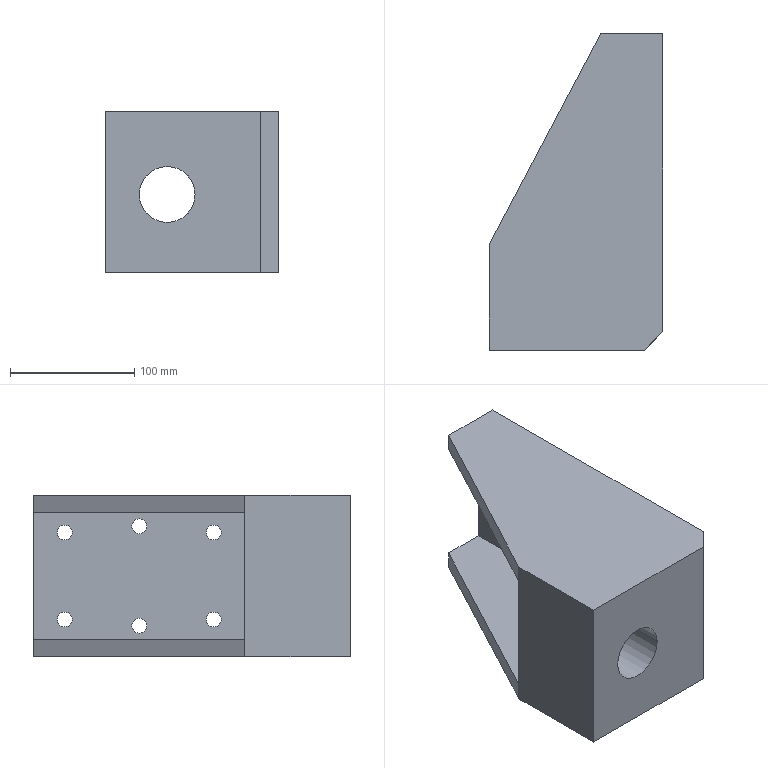Part | SolidWorks | features ICE 4, HoleWzd 2, Extrusion 1 | 1 solid | 27 faces | box 140 x 255 x 130 mm | volume 2115971 mm3 | cylinder 14 | plane 13 | commonest cylinder face diameters 12 x12 45 x2
STEP:
#1=CARTESIAN_POINT('',(-67.5,90.,63.));
#2=VERTEX_POINT('',#1);
#3=CARTESIAN_POINT('',(-112.5,90.,63.));
#4=VERTEX_POINT('',#3);
#5=CARTESIAN_POINT('',(-90.,90.,63.));
#6=DIRECTION('',(0.,1.,0.));
#7=DIRECTION('',(0.,0.,1.));
#8=AXIS2_PLACEMENT_3D('',#5,#6,#7);
#9=CIRCLE('',#8,22.5);
#10=EDGE_CURVE('',#2,#4,#9,.T.);
#11=ORIENTED_EDGE('',*,*,#10,.T.);
#12=CARTESIAN_POINT('',(-112.5,5.,63.));
#13=VERTEX_POINT('',#12);
#14=CARTESIAN_POINT('',(-112.5,260.001,63.));
#15=DIRECTION('',(0.,-1.,0.));
#16=VECTOR('',#15,1000.);
#17=LINE('',#14,#16);
#18=EDGE_CURVE('',#4,#13,#17,.T.);
#19=ORIENTED_EDGE('',*,*,#18,.T.);
#20=CARTESIAN_POINT('',(-67.5,5.,63.));
#21=VERTEX_POINT('',#20);
#22=CARTESIAN_POINT('',(-90.,5.,63.));
#23=DIRECTION('',(0.,1.,0.));
#24=DIRECTION('',(-1.,0.,0.));
#25=AXIS2_PLACEMENT_3D('',#22,#23,#24);
#26=CIRCLE('',#25,22.5);
#27=EDGE_CURVE('',#21,#13,#26,.T.);
#28=ORIENTED_EDGE('',*,*,#27,.F.);
#29=CARTESIAN_POINT('',(-67.5,260.001,63.));
#30=DIRECTION('',(0.,-1.,0.));
#31=VECTOR('',#30,1000.);
#32=LINE('',#29,#31);
#33=EDGE_CURVE('',#2,#21,#32,.T.);
#34=ORIENTED_EDGE('',*,*,#33,.F.);
#35=EDGE_LOOP('',(#11,#19,#28,#34));
#36=FACE_OUTER_BOUND('',#35,.T.);
#37=CARTESIAN_POINT('',(-90.,260.001,63.));
#38=DIRECTION('',(0.,-1.,0.));
#39=DIRECTION('',(1.,0.,0.));
#40=AXIS2_PLACEMENT_3D('',#37,#38,#39);
#41=CYLINDRICAL_SURFACE('',#40,22.5);
#42=ADVANCED_FACE('',(#36),#41,.F.);
#43=CARTESIAN_POINT('',(-16.,175.,99.));
#44=VERTEX_POINT('',#43);
#45=CARTESIAN_POINT('',(-16.,175.,111.));
#46=VERTEX_POINT('',#45);
#47=CARTESIAN_POINT('',(-16.,175.,105.));
#48=DIRECTION('',(-1.,0.,0.));
#49=DIRECTION('',(0.,-1.,0.));
#50=AXIS2_PLACEMENT_3D('',#47,#48,#49);
#51=CIRCLE('',#50,6.);
#52=EDGE_CURVE('',#44,#46,#51,.T.);
#53=ORIENTED_EDGE('',*,*,#52,.T.);
#54=CARTESIAN_POINT('',(0.,175.,111.));
#55=VERTEX_POINT('',#54);
#56=CARTESIAN_POINT('',(0.,175.,111.));
#57=DIRECTION('',(1.,0.,0.));
#58=VECTOR('',#57,1000.);
#59=LINE('',#56,#58);
#60=EDGE_CURVE('',#46,#55,#59,.T.);
#61=ORIENTED_EDGE('',*,*,#60,.T.);
#62=CARTESIAN_POINT('',(0.,175.,99.));
#63=VERTEX_POINT('',#62);
#64=CARTESIAN_POINT('',(0.,175.,105.));
#65=DIRECTION('',(1.,0.,0.));
#66=DIRECTION('',(0.,0.,-1.));
#67=AXIS2_PLACEMENT_3D('',#64,#65,#66);
#68=CIRCLE('',#67,6.);
#69=EDGE_CURVE('',#55,#63,#68,.T.);
#70=ORIENTED_EDGE('',*,*,#69,.T.);
#71=CARTESIAN_POINT('',(0.,175.,99.));
#72=DIRECTION('',(1.,0.,0.));
#73=VECTOR('',#72,1000.);
#74=LINE('',#71,#73);
#75=EDGE_CURVE('',#44,#63,#74,.T.);
#76=ORIENTED_EDGE('',*,*,#75,.F.);
#77=EDGE_LOOP('',(#53,#61,#70,#76));
#78=FACE_OUTER_BOUND('',#77,.T.);
#79=CARTESIAN_POINT('',(0.,175.,105.));
#80=DIRECTION('',(1.,0.,0.));
#81=DIRECTION('',(0.,0.,-1.));
#82=AXIS2_PLACEMENT_3D('',#79,#80,#81);
#83=CYLINDRICAL_SURFACE('',#82,6.);
#84=ADVANCED_FACE('',(#78),#83,.F.);
#85=CARTESIAN_POINT('',(-16.,175.,19.));
#86=VERTEX_POINT('',#85);
#87=CARTESIAN_POINT('',(-16.,175.,31.));
#88=VERTEX_POINT('',#87);
#89=CARTESIAN_POINT('',(-16.,175.,25.));
#90=DIRECTION('',(-1.,0.,0.));
#91=DIRECTION('',(0.,-1.,0.));
#92=AXIS2_PLACEMENT_3D('',#89,#90,#91);
#93=CIRCLE('',#92,6.);
#94=EDGE_CURVE('',#86,#88,#93,.T.);
#95=ORIENTED_EDGE('',*,*,#94,.T.);
#96=CARTESIAN_POINT('',(0.,175.,31.));
#97=VERTEX_POINT('',#96);
#98=CARTESIAN_POINT('',(0.,175.,31.));
#99=DIRECTION('',(1.,0.,0.));
#100=VECTOR('',#99,1000.);
#101=LINE('',#98,#100);
#102=EDGE_CURVE('',#88,#97,#101,.T.);
#103=ORIENTED_EDGE('',*,*,#102,.T.);
#104=CARTESIAN_POINT('',(0.,175.,19.));
#105=VERTEX_POINT('',#104);
#106=CARTESIAN_POINT('',(0.,175.,25.));
#107=DIRECTION('',(1.,0.,0.));
#108=DIRECTION('',(0.,0.,-1.));
#109=AXIS2_PLACEMENT_3D('',#106,#107,#108);
#110=CIRCLE('',#109,6.);
#111=EDGE_CURVE('',#97,#105,#110,.T.);
#112=ORIENTED_EDGE('',*,*,#111,.T.);
#113=CARTESIAN_POINT('',(0.,175.,19.));
#114=DIRECTION('',(1.,0.,0.));
#115=VECTOR('',#114,1000.);
#116=LINE('',#113,#115);
#117=EDGE_CURVE('',#86,#105,#116,.T.);
#118=ORIENTED_EDGE('',*,*,#117,.F.);
#119=EDGE_LOOP('',(#95,#103,#112,#118));
#120=FACE_OUTER_BOUND('',#119,.T.);
#121=CARTESIAN_POINT('',(0.,175.,25.));
#122=DIRECTION('',(1.,0.,0.));
#123=DIRECTION('',(0.,0.,-1.));
#124=AXIS2_PLACEMENT_3D('',#121,#122,#123);
#125=CYLINDRICAL_SURFACE('',#124,6.);
#126=ADVANCED_FACE('',(#120),#125,.F.);
#127=CARTESIAN_POINT('',(-16.,235.,94.));
#128=VERTEX_POINT('',#127);
#129=CARTESIAN_POINT('',(-16.,235.,106.));
#130=VERTEX_POINT('',#129);
#131=CARTESIAN_POINT('',(-16.,235.,100.));
#132=DIRECTION('',(-1.,0.,0.));
#133=DIRECTION('',(0.,-1.,0.));
#134=AXIS2_PLACEMENT_3D('',#131,#132,#133);
#135=CIRCLE('',#134,6.);
#136=EDGE_CURVE('',#128,#130,#135,.T.);
#137=ORIENTED_EDGE('',*,*,#136,.T.);
#138=CARTESIAN_POINT('',(0.,235.,106.));
#139=VERTEX_POINT('',#138);
#140=CARTESIAN_POINT('',(0.,235.,106.));
#141=DIRECTION('',(1.,0.,0.));
#142=VECTOR('',#141,1000.);
#143=LINE('',#140,#142);
#144=EDGE_CURVE('',#130,#139,#143,.T.);
#145=ORIENTED_EDGE('',*,*,#144,.T.);
#146=CARTESIAN_POINT('',(0.,235.,94.));
#147=VERTEX_POINT('',#146);
#148=CARTESIAN_POINT('',(0.,235.,100.));
#149=DIRECTION('',(1.,0.,0.));
#150=DIRECTION('',(0.,0.,-1.));
#151=AXIS2_PLACEMENT_3D('',#148,#149,#150);
#152=CIRCLE('',#151,6.);
#153=EDGE_CURVE('',#139,#147,#152,.T.);
#154=ORIENTED_EDGE('',*,*,#153,.T.);
#155=CARTESIAN_POINT('',(0.,235.,94.));
#156=DIRECTION('',(1.,0.,0.));
#157=VECTOR('',#156,1000.);
#158=LINE('',#155,#157);
#159=EDGE_CURVE('',#128,#147,#158,.T.);
#160=ORIENTED_EDGE('',*,*,#159,.F.);
#161=EDGE_LOOP('',(#137,#145,#154,#160));
#162=FACE_OUTER_BOUND('',#161,.T.);
#163=CARTESIAN_POINT('',(0.,235.,100.));
#164=DIRECTION('',(1.,0.,0.));
#165=DIRECTION('',(0.,0.,-1.));
#166=AXIS2_PLACEMENT_3D('',#163,#164,#165);
#167=CYLINDRICAL_SURFACE('',#166,6.);
#168=ADVANCED_FACE('',(#162),#167,.F.);
#169=CARTESIAN_POINT('',(-16.,235.,24.));
#170=VERTEX_POINT('',#169);
#171=CARTESIAN_POINT('',(-16.,235.,36.));
#172=VERTEX_POINT('',#171);
#173=CARTESIAN_POINT('',(-16.,235.,30.));
#174=DIRECTION('',(-1.,0.,0.));
#175=DIRECTION('',(0.,-1.,0.));
#176=AXIS2_PLACEMENT_3D('',#173,#174,#175);
#177=CIRCLE('',#176,6.);
#178=EDGE_CURVE('',#170,#172,#177,.T.);
#179=ORIENTED_EDGE('',*,*,#178,.T.);
#180=CARTESIAN_POINT('',(0.,235.,36.));
#181=VERTEX_POINT('',#180);
#182=CARTESIAN_POINT('',(0.,235.,36.));
#183=DIRECTION('',(1.,0.,0.));
#184=VECTOR('',#183,1000.);
#185=LINE('',#182,#184);
#186=EDGE_CURVE('',#172,#181,#185,.T.);
#187=ORIENTED_EDGE('',*,*,#186,.T.);
#188=CARTESIAN_POINT('',(0.,235.,24.));
#189=VERTEX_POINT('',#188);
#190=CARTESIAN_POINT('',(0.,235.,30.));
#191=DIRECTION('',(1.,0.,0.));
#192=DIRECTION('',(0.,0.,-1.));
#193=AXIS2_PLACEMENT_3D('',#190,#191,#192);
#194=CIRCLE('',#193,6.);
#195=EDGE_CURVE('',#181,#189,#194,.T.);
#196=ORIENTED_EDGE('',*,*,#195,.T.);
#197=CARTESIAN_POINT('',(0.,235.,24.));
#198=DIRECTION('',(1.,0.,0.));
#199=VECTOR('',#198,1000.);
#200=LINE('',#197,#199);
#201=EDGE_CURVE('',#170,#189,#200,.T.);
#202=ORIENTED_EDGE('',*,*,#201,.F.);
#203=EDGE_LOOP('',(#179,#187,#196,#202));
#204=FACE_OUTER_BOUND('',#203,.T.);
#205=CARTESIAN_POINT('',(0.,235.,30.));
#206=DIRECTION('',(1.,0.,0.));
#207=DIRECTION('',(0.,0.,-1.));
#208=AXIS2_PLACEMENT_3D('',#205,#206,#207);
#209=CYLINDRICAL_SURFACE('',#208,6.);
#210=ADVANCED_FACE('',(#204),#209,.F.);
#211=CARTESIAN_POINT('',(-16.,115.,94.));
#212=VERTEX_POINT('',#211);
#213=CARTESIAN_POINT('',(-16.,115.,106.));
#214=VERTEX_POINT('',#213);
#215=CARTESIAN_POINT('',(-16.,115.,100.));
#216=DIRECTION('',(-1.,0.,0.));
#217=DIRECTION('',(0.,-1.,0.));
#218=AXIS2_PLACEMENT_3D('',#215,#216,#217);
#219=CIRCLE('',#218,6.);
#220=EDGE_CURVE('',#212,#214,#219,.T.);
#221=ORIENTED_EDGE('',*,*,#220,.T.);
#222=CARTESIAN_POINT('',(0.,115.,106.));
#223=VERTEX_POINT('',#222);
#224=CARTESIAN_POINT('',(0.,115.,106.));
#225=DIRECTION('',(1.,0.,0.));
#226=VECTOR('',#225,1000.);
#227=LINE('',#224,#226);
#228=EDGE_CURVE('',#214,#223,#227,.T.);
#229=ORIENTED_EDGE('',*,*,#228,.T.);
#230=CARTESIAN_POINT('',(0.,115.,94.));
#231=VERTEX_POINT('',#230);
#232=CARTESIAN_POINT('',(0.,115.,100.));
#233=DIRECTION('',(1.,0.,0.));
#234=DIRECTION('',(0.,0.,-1.));
#235=AXIS2_PLACEMENT_3D('',#232,#233,#234);
#236=CIRCLE('',#235,6.);
#237=EDGE_CURVE('',#223,#231,#236,.T.);
#238=ORIENTED_EDGE('',*,*,#237,.T.);
#239=CARTESIAN_POINT('',(0.,115.,94.));
#240=DIRECTION('',(1.,0.,0.));
#241=VECTOR('',#240,1000.);
#242=LINE('',#239,#241);
#243=EDGE_CURVE('',#212,#231,#242,.T.);
#244=ORIENTED_EDGE('',*,*,#243,.F.);
#245=EDGE_LOOP('',(#221,#229,#238,#244));
#246=FACE_OUTER_BOUND('',#245,.T.);
#247=CARTESIAN_POINT('',(0.,115.,100.));
#248=DIRECTION('',(1.,0.,0.));
#249=DIRECTION('',(0.,0.,-1.));
#250=AXIS2_PLACEMENT_3D('',#247,#248,#249);
#251=CYLINDRICAL_SURFACE('',#250,6.);
#252=ADVANCED_FACE('',(#246),#251,.F.);
#253=CARTESIAN_POINT('',(-16.,115.,24.));
#254=VERTEX_POINT('',#253);
#255=CARTESIAN_POINT('',(-16.,115.,36.));
#256=VERTEX_POINT('',#255);
#257=CARTESIAN_POINT('',(-16.,115.,30.));
#258=DIRECTION('',(-1.,0.,0.));
#259=DIRECTION('',(0.,-1.,0.));
#260=AXIS2_PLACEMENT_3D('',#257,#258,#259);
#261=CIRCLE('',#260,6.);
#262=EDGE_CURVE('',#254,#256,#261,.T.);
#263=ORIENTED_EDGE('',*,*,#262,.T.);
#264=CARTESIAN_POINT('',(0.,115.,36.));
#265=VERTEX_POINT('',#264);
#266=CARTESIAN_POINT('',(0.,115.,36.));
#267=DIRECTION('',(1.,0.,0.));
#268=VECTOR('',#267,1000.);
#269=LINE('',#266,#268);
#270=EDGE_CURVE('',#256,#265,#269,.T.);
#271=ORIENTED_EDGE('',*,*,#270,.T.);
#272=CARTESIAN_POINT('',(0.,115.,24.));
#273=VERTEX_POINT('',#272);
#274=CARTESIAN_POINT('',(0.,115.,30.));
#275=DIRECTION('',(1.,0.,0.));
#276=DIRECTION('',(0.,0.,-1.));
#277=AXIS2_PLACEMENT_3D('',#274,#275,#276);
#278=CIRCLE('',#277,6.);
#279=EDGE_CURVE('',#265,#273,#278,.T.);
#280=ORIENTED_EDGE('',*,*,#279,.T.);
#281=CARTESIAN_POINT('',(0.,115.,24.));
#282=DIRECTION('',(1.,0.,0.));
#283=VECTOR('',#282,1000.);
#284=LINE('',#281,#283);
#285=EDGE_CURVE('',#254,#273,#284,.T.);
#286=ORIENTED_EDGE('',*,*,#285,.F.);
#287=EDGE_LOOP('',(#263,#271,#280,#286));
#288=FACE_OUTER_BOUND('',#287,.T.);
#289=CARTESIAN_POINT('',(0.,115.,30.));
#290=DIRECTION('',(1.,0.,0.));
#291=DIRECTION('',(0.,0.,-1.));
#292=AXIS2_PLACEMENT_3D('',#289,#290,#291);
#293=CYLINDRICAL_SURFACE('',#292,6.);
#294=ADVANCED_FACE('',(#288),#293,.F.);
#295=CARTESIAN_POINT('',(0.,175.,105.));
#296=DIRECTION('',(1.,0.,0.));
#297=DIRECTION('',(0.,0.,-1.));
#298=AXIS2_PLACEMENT_3D('',#295,#296,#297);
#299=CIRCLE('',#298,6.);
#300=EDGE_CURVE('',#63,#55,#299,.T.);
#301=ORIENTED_EDGE('',*,*,#300,.F.);
#302=ORIENTED_EDGE('',*,*,#69,.F.);
#303=EDGE_LOOP('',(#301,#302));
#304=FACE_BOUND('',#303,.T.);
#305=CARTESIAN_POINT('',(0.,235.,100.));
#306=DIRECTION('',(1.,0.,0.));
#307=DIRECTION('',(0.,0.,-1.));
#308=AXIS2_PLACEMENT_3D('',#305,#306,#307);
#309=CIRCLE('',#308,6.);
#310=EDGE_CURVE('',#147,#139,#309,.T.);
#311=ORIENTED_EDGE('',*,*,#310,.F.);
#312=ORIENTED_EDGE('',*,*,#153,.F.);
#313=EDGE_LOOP('',(#311,#312));
#314=FACE_BOUND('',#313,.T.);
#315=CARTESIAN_POINT('',(0.,235.,30.));
#316=DIRECTION('',(1.,0.,0.));
#317=DIRECTION('',(0.,0.,-1.));
#318=AXIS2_PLACEMENT_3D('',#315,#316,#317);
#319=CIRCLE('',#318,6.);
#320=EDGE_CURVE('',#189,#181,#319,.T.);
#321=ORIENTED_EDGE('',*,*,#320,.F.);
#322=ORIENTED_EDGE('',*,*,#195,.F.);
#323=EDGE_LOOP('',(#321,#322));
#324=FACE_BOUND('',#323,.T.);
#325=CARTESIAN_POINT('',(0.,115.,100.));
#326=DIRECTION('',(1.,0.,0.));
#327=DIRECTION('',(0.,0.,-1.));
#328=AXIS2_PLACEMENT_3D('',#325,#326,#327);
#329=CIRCLE('',#328,6.);
#330=EDGE_CURVE('',#231,#223,#329,.T.);
#331=ORIENTED_EDGE('',*,*,#330,.F.);
#332=ORIENTED_EDGE('',*,*,#237,.F.);
#333=EDGE_LOOP('',(#331,#332));
#334=FACE_BOUND('',#333,.T.);
#335=CARTESIAN_POINT('',(0.,115.,30.));
#336=DIRECTION('',(1.,0.,0.));
#337=DIRECTION('',(0.,0.,-1.));
#338=AXIS2_PLACEMENT_3D('',#335,#336,#337);
#339=CIRCLE('',#338,6.);
#340=EDGE_CURVE('',#273,#265,#339,.T.);
#341=ORIENTED_EDGE('',*,*,#340,.F.);
#342=ORIENTED_EDGE('',*,*,#279,.F.);
#343=EDGE_LOOP('',(#341,#342));
#344=FACE_BOUND('',#343,.T.);
#345=CARTESIAN_POINT('',(0.,20.,130.));
#346=VERTEX_POINT('',#345);
#347=CARTESIAN_POINT('',(0.,260.,130.));
#348=VERTEX_POINT('',#347);
#349=CARTESIAN_POINT('',(0.,260.,130.));
#350=DIRECTION('',(0.,1.,0.));
#351=VECTOR('',#350,1000.);
#352=LINE('',#349,#351);
#353=EDGE_CURVE('',#346,#348,#352,.T.);
#354=ORIENTED_EDGE('',*,*,#353,.F.);
#355=CARTESIAN_POINT('',(0.,20.,0.));
#356=VERTEX_POINT('',#355);
#357=CARTESIAN_POINT('',(0.,20.,0.));
#358=DIRECTION('',(0.,0.,1.));
#359=VECTOR('',#358,1000.);
#360=LINE('',#357,#359);
#361=EDGE_CURVE('',#356,#346,#360,.T.);
#362=ORIENTED_EDGE('',*,*,#361,.F.);
#363=CARTESIAN_POINT('',(0.,260.,0.));
#364=VERTEX_POINT('',#363);
#365=CARTESIAN_POINT('',(0.,260.,0.));
#366=DIRECTION('',(0.,1.,0.));
#367=VECTOR('',#366,1000.);
#368=LINE('',#365,#367);
#369=EDGE_CURVE('',#356,#364,#368,.T.);
#370=ORIENTED_EDGE('',*,*,#369,.T.);
#371=CARTESIAN_POINT('',(0.,260.,130.));
#372=DIRECTION('',(0.,0.,-1.));
#373=VECTOR('',#372,1000.);
#374=LINE('',#371,#373);
#375=EDGE_CURVE('',#348,#364,#374,.T.);
#376=ORIENTED_EDGE('',*,*,#375,.F.);
#377=EDGE_LOOP('',(#354,#362,#370,#376));
#378=FACE_OUTER_BOUND('',#377,.T.);
#379=CARTESIAN_POINT('',(0.,175.,25.));
#380=DIRECTION('',(1.,0.,0.));
#381=DIRECTION('',(0.,0.,-1.));
#382=AXIS2_PLACEMENT_3D('',#379,#380,#381);
#383=CIRCLE('',#382,6.);
#384=EDGE_CURVE('',#105,#97,#383,.T.);
#385=ORIENTED_EDGE('',*,*,#384,.F.);
#386=ORIENTED_EDGE('',*,*,#111,.F.);
#387=EDGE_LOOP('',(#385,#386));
#388=FACE_BOUND('',#387,.T.);
#389=CARTESIAN_POINT('',(0.,260.,130.));
#390=DIRECTION('',(-1.,0.,0.));
#391=DIRECTION('',(0.,-1.,0.));
#392=AXIS2_PLACEMENT_3D('',#389,#390,#391);
#393=PLANE('',#392);
#394=ADVANCED_FACE('',(#304,#314,#324,#334,#344,#378,#388),#393,.F.);
#395=CARTESIAN_POINT('',(-16.,260.,14.));
#396=VERTEX_POINT('',#395);
#397=CARTESIAN_POINT('',(-50.,260.,14.));
#398=VERTEX_POINT('',#397);
#399=CARTESIAN_POINT('',(198.252,260.,14.));
#400=DIRECTION('',(-1.,0.,0.));
#401=VECTOR('',#400,1000.);
#402=LINE('',#399,#401);
#403=EDGE_CURVE('',#396,#398,#402,.T.);
#404=ORIENTED_EDGE('',*,*,#403,.F.);
#405=CARTESIAN_POINT('',(-16.,260.,116.));
#406=VERTEX_POINT('',#405);
#407=CARTESIAN_POINT('',(-16.,260.,116.));
#408=DIRECTION('',(0.,0.,-1.));
#409=VECTOR('',#408,1000.);
#410=LINE('',#407,#409);
#411=EDGE_CURVE('',#406,#396,#410,.T.);
#412=ORIENTED_EDGE('',*,*,#411,.F.);
#413=CARTESIAN_POINT('',(-50.,260.,116.));
#414=VERTEX_POINT('',#413);
#415=CARTESIAN_POINT('',(198.252,260.,116.));
#416=DIRECTION('',(-1.,0.,0.));
#417=VECTOR('',#416,1000.);
#418=LINE('',#415,#417);
#419=EDGE_CURVE('',#406,#414,#418,.T.);
#420=ORIENTED_EDGE('',*,*,#419,.T.);
#421=CARTESIAN_POINT('',(-50.,260.,130.));
#422=VERTEX_POINT('',#421);
#423=CARTESIAN_POINT('',(-50.,260.,130.));
#424=DIRECTION('',(0.,0.,-1.));
#425=VECTOR('',#424,1000.);
#426=LINE('',#423,#425);
#427=EDGE_CURVE('',#422,#414,#426,.T.);
#428=ORIENTED_EDGE('',*,*,#427,.F.);
#429=CARTESIAN_POINT('',(-50.,260.,130.));
#430=DIRECTION('',(-1.,0.,0.));
#431=VECTOR('',#430,1000.);
#432=LINE('',#429,#431);
#433=EDGE_CURVE('',#348,#422,#432,.T.);
#434=ORIENTED_EDGE('',*,*,#433,.F.);
#435=ORIENTED_EDGE('',*,*,#375,.T.);
#436=CARTESIAN_POINT('',(-50.,260.,0.));
#437=VERTEX_POINT('',#436);
#438=CARTESIAN_POINT('',(-50.,260.,0.));
#439=DIRECTION('',(-1.,0.,0.));
#440=VECTOR('',#439,1000.);
#441=LINE('',#438,#440);
#442=EDGE_CURVE('',#364,#437,#441,.T.);
#443=ORIENTED_EDGE('',*,*,#442,.T.);
#444=CARTESIAN_POINT('',(-50.,260.,130.));
#445=DIRECTION('',(0.,0.,-1.));
#446=VECTOR('',#445,1000.);
#447=LINE('',#444,#446);
#448=EDGE_CURVE('',#398,#437,#447,.T.);
#449=ORIENTED_EDGE('',*,*,#448,.F.);
#450=EDGE_LOOP('',(#404,#412,#420,#428,#434,#435,#443,#449));
#451=FACE_OUTER_BOUND('',#450,.T.);
#452=CARTESIAN_POINT('',(-50.,260.,130.));
#453=DIRECTION('',(0.,-1.,0.));
#454=DIRECTION('',(0.,0.,-1.));
#455=AXIS2_PLACEMENT_3D('',#452,#453,#454);
#456=PLANE('',#455);
#457=ADVANCED_FACE('',(#451),#456,.F.);
#458=CARTESIAN_POINT('',(-140.,90.,14.));
#459=VERTEX_POINT('',#458);
#460=CARTESIAN_POINT('',(-140.,90.,14.));
#461=DIRECTION('',(-0.4679,-0.8838,0.));
#462=VECTOR('',#461,1000.);
#463=LINE('',#460,#462);
#464=EDGE_CURVE('',#398,#459,#463,.T.);
#465=ORIENTED_EDGE('',*,*,#464,.F.);
#466=ORIENTED_EDGE('',*,*,#448,.T.);
#467=CARTESIAN_POINT('',(-140.,90.,0.));
#468=VERTEX_POINT('',#467);
#469=CARTESIAN_POINT('',(-140.,90.,0.));
#470=DIRECTION('',(-0.4679,-0.8838,0.));
#471=VECTOR('',#470,1000.);
#472=LINE('',#469,#471);
#473=EDGE_CURVE('',#437,#468,#472,.T.);
#474=ORIENTED_EDGE('',*,*,#473,.T.);
#475=CARTESIAN_POINT('',(-140.,90.,130.));
#476=DIRECTION('',(0.,0.,-1.));
#477=VECTOR('',#476,1000.);
#478=LINE('',#475,#477);
#479=EDGE_CURVE('',#459,#468,#478,.T.);
#480=ORIENTED_EDGE('',*,*,#479,.F.);
#481=EDGE_LOOP('',(#465,#466,#474,#480));
#482=FACE_OUTER_BOUND('',#481,.T.);
#483=CARTESIAN_POINT('',(-140.,90.,130.));
#484=DIRECTION('',(0.8838,-0.4679,0.));
#485=DIRECTION('',(0.4679,0.8838,0.));
#486=AXIS2_PLACEMENT_3D('',#483,#484,#485);
#487=PLANE('',#486);
#488=ADVANCED_FACE('',(#482),#487,.F.);
#489=CARTESIAN_POINT('',(-140.,90.,116.));
#490=VERTEX_POINT('',#489);
#491=CARTESIAN_POINT('',(-140.,90.,116.));
#492=DIRECTION('',(0.4679,0.8838,0.));
#493=VECTOR('',#492,1000.);
#494=LINE('',#491,#493);
#495=EDGE_CURVE('',#490,#414,#494,.T.);
#496=ORIENTED_EDGE('',*,*,#495,.F.);
#497=CARTESIAN_POINT('',(-140.,90.,130.));
#498=VERTEX_POINT('',#497);
#499=CARTESIAN_POINT('',(-140.,90.,130.));
#500=DIRECTION('',(0.,0.,-1.));
#501=VECTOR('',#500,1000.);
#502=LINE('',#499,#501);
#503=EDGE_CURVE('',#498,#490,#502,.T.);
#504=ORIENTED_EDGE('',*,*,#503,.F.);
#505=CARTESIAN_POINT('',(-140.,90.,130.));
#506=DIRECTION('',(-0.4679,-0.8838,0.));
#507=VECTOR('',#506,1000.);
#508=LINE('',#505,#507);
#509=EDGE_CURVE('',#422,#498,#508,.T.);
#510=ORIENTED_EDGE('',*,*,#509,.F.);
#511=ORIENTED_EDGE('',*,*,#427,.T.);
#512=EDGE_LOOP('',(#496,#504,#510,#511));
#513=FACE_OUTER_BOUND('',#512,.T.);
#514=CARTESIAN_POINT('',(-140.,90.,130.));
#515=DIRECTION('',(0.8838,-0.4679,0.));
#516=DIRECTION('',(0.4679,0.8838,0.));
#517=AXIS2_PLACEMENT_3D('',#514,#515,#516);
#518=PLANE('',#517);
#519=ADVANCED_FACE('',(#513),#518,.F.);
#520=CARTESIAN_POINT('',(-140.,5.,0.));
#521=VERTEX_POINT('',#520);
#522=CARTESIAN_POINT('',(-140.,0.,0.));
#523=DIRECTION('',(0.,-1.,0.));
#524=VECTOR('',#523,1000.);
#525=LINE('',#522,#524);
#526=EDGE_CURVE('',#468,#521,#525,.T.);
#527=ORIENTED_EDGE('',*,*,#526,.T.);
#528=CARTESIAN_POINT('',(-140.,5.,130.));
#529=VERTEX_POINT('',#528);
#530=CARTESIAN_POINT('',(-140.,5.,0.));
#531=DIRECTION('',(0.,0.,1.));
#532=VECTOR('',#531,1000.);
#533=LINE('',#530,#532);
#534=EDGE_CURVE('',#521,#529,#533,.T.);
#535=ORIENTED_EDGE('',*,*,#534,.T.);
#536=CARTESIAN_POINT('',(-140.,0.,130.));
#537=DIRECTION('',(0.,-1.,0.));
#538=VECTOR('',#537,1000.);
#539=LINE('',#536,#538);
#540=EDGE_CURVE('',#498,#529,#539,.T.);
#541=ORIENTED_EDGE('',*,*,#540,.F.);
#542=ORIENTED_EDGE('',*,*,#503,.T.);
#543=CARTESIAN_POINT('',(-140.,90.,116.));
#544=DIRECTION('',(0.,0.,-1.));
#545=VECTOR('',#544,1000.);
#546=LINE('',#543,#545);
#547=EDGE_CURVE('',#490,#459,#546,.T.);
#548=ORIENTED_EDGE('',*,*,#547,.T.);
#549=ORIENTED_EDGE('',*,*,#479,.T.);
#550=EDGE_LOOP('',(#527,#535,#541,#542,#548,#549));
#551=FACE_OUTER_BOUND('',#550,.T.);
#552=CARTESIAN_POINT('',(-140.,0.,130.));
#553=DIRECTION('',(1.,0.,0.));
#554=DIRECTION('',(0.,0.,-1.));
#555=AXIS2_PLACEMENT_3D('',#552,#553,#554);
#556=PLANE('',#555);
#557=ADVANCED_FACE('',(#551),#556,.F.);
#558=CARTESIAN_POINT('',(-15.,5.,130.));
#559=VERTEX_POINT('',#558);
#560=CARTESIAN_POINT('',(0.,5.,130.));
#561=DIRECTION('',(-1.,0.,0.));
#562=VECTOR('',#561,1000.);
#563=LINE('',#560,#562);
#564=EDGE_CURVE('',#559,#529,#563,.T.);
#565=ORIENTED_EDGE('',*,*,#564,.F.);
#566=CARTESIAN_POINT('',(0.,20.,130.));
#567=DIRECTION('',(-0.7071,-0.7071,0.));
#568=VECTOR('',#567,1000.);
#569=LINE('',#566,#568);
#570=EDGE_CURVE('',#346,#559,#569,.T.);
#571=ORIENTED_EDGE('',*,*,#570,.F.);
#572=ORIENTED_EDGE('',*,*,#353,.T.);
#573=ORIENTED_EDGE('',*,*,#433,.T.);
#574=ORIENTED_EDGE('',*,*,#509,.T.);
#575=ORIENTED_EDGE('',*,*,#540,.T.);
#576=EDGE_LOOP('',(#565,#571,#572,#573,#574,#575));
#577=FACE_OUTER_BOUND('',#576,.T.);
#578=CARTESIAN_POINT('',(0.,0.,130.));
#579=DIRECTION('',(0.,0.,-1.));
#580=DIRECTION('',(-1.,0.,0.));
#581=AXIS2_PLACEMENT_3D('',#578,#579,#580);
#582=PLANE('',#581);
#583=ADVANCED_FACE('',(#577),#582,.F.);
#584=CARTESIAN_POINT('',(-15.,5.,0.));
#585=VERTEX_POINT('',#584);
#586=CARTESIAN_POINT('',(0.,20.,0.));
#587=DIRECTION('',(-0.7071,-0.7071,0.));
#588=VECTOR('',#587,1000.);
#589=LINE('',#586,#588);
#590=EDGE_CURVE('',#356,#585,#589,.T.);
#591=ORIENTED_EDGE('',*,*,#590,.T.);
#592=CARTESIAN_POINT('',(0.,5.,0.));
#593=DIRECTION('',(-1.,0.,0.));
#594=VECTOR('',#593,1000.);
#595=LINE('',#592,#594);
#596=EDGE_CURVE('',#585,#521,#595,.T.);
#597=ORIENTED_EDGE('',*,*,#596,.T.);
#598=ORIENTED_EDGE('',*,*,#526,.F.);
#599=ORIENTED_EDGE('',*,*,#473,.F.);
#600=ORIENTED_EDGE('',*,*,#442,.F.);
#601=ORIENTED_EDGE('',*,*,#369,.F.);
#602=EDGE_LOOP('',(#591,#597,#598,#599,#600,#601));
#603=FACE_OUTER_BOUND('',#602,.T.);
#604=CARTESIAN_POINT('',(0.,0.,0.));
#605=DIRECTION('',(0.,0.,-1.));
#606=DIRECTION('',(-1.,0.,0.));
#607=AXIS2_PLACEMENT_3D('',#604,#605,#606);
#608=PLANE('',#607);
#609=ADVANCED_FACE('',(#603),#608,.T.);
#610=ORIENTED_EDGE('',*,*,#27,.T.);
#611=CARTESIAN_POINT('',(-90.,5.,63.));
#612=DIRECTION('',(0.,1.,0.));
#613=DIRECTION('',(-1.,0.,0.));
#614=AXIS2_PLACEMENT_3D('',#611,#612,#613);
#615=CIRCLE('',#614,22.5);
#616=EDGE_CURVE('',#13,#21,#615,.T.);
#617=ORIENTED_EDGE('',*,*,#616,.T.);
#618=EDGE_LOOP('',(#610,#617));
#619=FACE_BOUND('',#618,.T.);
#620=ORIENTED_EDGE('',*,*,#596,.F.);
#621=CARTESIAN_POINT('',(-15.,5.,0.));
#622=DIRECTION('',(0.,0.,1.));
#623=VECTOR('',#622,1000.);
#624=LINE('',#621,#623);
#625=EDGE_CURVE('',#585,#559,#624,.T.);
#626=ORIENTED_EDGE('',*,*,#625,.T.);
#627=ORIENTED_EDGE('',*,*,#564,.T.);
#628=ORIENTED_EDGE('',*,*,#534,.F.);
#629=EDGE_LOOP('',(#620,#626,#627,#628));
#630=FACE_OUTER_BOUND('',#629,.T.);
#631=CARTESIAN_POINT('',(0.,5.,0.));
#632=DIRECTION('',(0.,1.,0.));
#633=DIRECTION('',(-1.,0.,0.));
#634=AXIS2_PLACEMENT_3D('',#631,#632,#633);
#635=PLANE('',#634);
#636=ADVANCED_FACE('',(#619,#630),#635,.F.);
#637=ORIENTED_EDGE('',*,*,#464,.T.);
#638=CARTESIAN_POINT('',(-16.,90.,14.));
#639=VERTEX_POINT('',#638);
#640=CARTESIAN_POINT('',(198.252,90.,14.));
#641=DIRECTION('',(-1.,0.,0.));
#642=VECTOR('',#641,1000.);
#643=LINE('',#640,#642);
#644=EDGE_CURVE('',#639,#459,#643,.T.);
#645=ORIENTED_EDGE('',*,*,#644,.F.);
#646=CARTESIAN_POINT('',(-16.,260.,14.));
#647=DIRECTION('',(0.,-1.,0.));
#648=VECTOR('',#647,1000.);
#649=LINE('',#646,#648);
#650=EDGE_CURVE('',#396,#639,#649,.T.);
#651=ORIENTED_EDGE('',*,*,#650,.F.);
#652=ORIENTED_EDGE('',*,*,#403,.T.);
#653=EDGE_LOOP('',(#637,#645,#651,#652));
#654=FACE_OUTER_BOUND('',#653,.T.);
#655=CARTESIAN_POINT('',(198.252,260.,14.));
#656=DIRECTION('',(0.,0.,1.));
#657=DIRECTION('',(0.,-1.,0.));
#658=AXIS2_PLACEMENT_3D('',#655,#656,#657);
#659=PLANE('',#658);
#660=ADVANCED_FACE('',(#654),#659,.T.);
#661=ORIENTED_EDGE('',*,*,#495,.T.);
#662=ORIENTED_EDGE('',*,*,#419,.F.);
#663=CARTESIAN_POINT('',(-16.,90.,116.));
#664=VERTEX_POINT('',#663);
#665=CARTESIAN_POINT('',(-16.,260.,116.));
#666=DIRECTION('',(0.,1.,0.));
#667=VECTOR('',#666,1000.);
#668=LINE('',#665,#667);
#669=EDGE_CURVE('',#664,#406,#668,.T.);
#670=ORIENTED_EDGE('',*,*,#669,.F.);
#671=CARTESIAN_POINT('',(198.252,90.,116.));
#672=DIRECTION('',(-1.,0.,0.));
#673=VECTOR('',#672,1000.);
#674=LINE('',#671,#673);
#675=EDGE_CURVE('',#664,#490,#674,.T.);
#676=ORIENTED_EDGE('',*,*,#675,.T.);
#677=EDGE_LOOP('',(#661,#662,#670,#676));
#678=FACE_OUTER_BOUND('',#677,.T.);
#679=CARTESIAN_POINT('',(198.252,260.,116.));
#680=DIRECTION('',(0.,0.,-1.));
#681=DIRECTION('',(0.,1.,0.));
#682=AXIS2_PLACEMENT_3D('',#679,#680,#681);
#683=PLANE('',#682);
#684=ADVANCED_FACE('',(#678),#683,.T.);
#685=ORIENTED_EDGE('',*,*,#10,.F.);
#686=CARTESIAN_POINT('',(-90.,90.,63.));
#687=DIRECTION('',(0.,1.,0.));
#688=DIRECTION('',(0.,0.,1.));
#689=AXIS2_PLACEMENT_3D('',#686,#687,#688);
#690=CIRCLE('',#689,22.5);
#691=EDGE_CURVE('',#4,#2,#690,.T.);
#692=ORIENTED_EDGE('',*,*,#691,.F.);
#693=EDGE_LOOP('',(#685,#692));
#694=FACE_BOUND('',#693,.T.);
#695=ORIENTED_EDGE('',*,*,#644,.T.);
#696=ORIENTED_EDGE('',*,*,#547,.F.);
#697=ORIENTED_EDGE('',*,*,#675,.F.);
#698=CARTESIAN_POINT('',(-16.,90.,116.));
#699=DIRECTION('',(0.,0.,1.));
#700=VECTOR('',#699,1000.);
#701=LINE('',#698,#700);
#702=EDGE_CURVE('',#639,#664,#701,.T.);
#703=ORIENTED_EDGE('',*,*,#702,.F.);
#704=EDGE_LOOP('',(#695,#696,#697,#703));
#705=FACE_OUTER_BOUND('',#704,.T.);
#706=CARTESIAN_POINT('',(198.252,90.,116.));
#707=DIRECTION('',(0.,1.,0.));
#708=DIRECTION('',(0.,0.,1.));
#709=AXIS2_PLACEMENT_3D('',#706,#707,#708);
#710=PLANE('',#709);
#711=ADVANCED_FACE('',(#694,#705),#710,.T.);
#712=ORIENTED_EDGE('',*,*,#52,.F.);
#713=CARTESIAN_POINT('',(-16.,175.,105.));
#714=DIRECTION('',(-1.,0.,0.));
#715=DIRECTION('',(0.,-1.,0.));
#716=AXIS2_PLACEMENT_3D('',#713,#714,#715);
#717=CIRCLE('',#716,6.);
#718=EDGE_CURVE('',#46,#44,#717,.T.);
#719=ORIENTED_EDGE('',*,*,#718,.F.);
#720=EDGE_LOOP('',(#712,#719));
#721=FACE_BOUND('',#720,.T.);
#722=ORIENTED_EDGE('',*,*,#94,.F.);
#723=CARTESIAN_POINT('',(-16.,175.,25.));
#724=DIRECTION('',(-1.,0.,0.));
#725=DIRECTION('',(0.,-1.,0.));
#726=AXIS2_PLACEMENT_3D('',#723,#724,#725);
#727=CIRCLE('',#726,6.);
#728=EDGE_CURVE('',#88,#86,#727,.T.);
#729=ORIENTED_EDGE('',*,*,#728,.F.);
#730=EDGE_LOOP('',(#722,#729));
#731=FACE_BOUND('',#730,.T.);
#732=ORIENTED_EDGE('',*,*,#136,.F.);
#733=CARTESIAN_POINT('',(-16.,235.,100.));
#734=DIRECTION('',(-1.,0.,0.));
#735=DIRECTION('',(0.,-1.,0.));
#736=AXIS2_PLACEMENT_3D('',#733,#734,#735);
#737=CIRCLE('',#736,6.);
#738=EDGE_CURVE('',#130,#128,#737,.T.);
#739=ORIENTED_EDGE('',*,*,#738,.F.);
#740=EDGE_LOOP('',(#732,#739));
#741=FACE_BOUND('',#740,.T.);
#742=ORIENTED_EDGE('',*,*,#178,.F.);
#743=CARTESIAN_POINT('',(-16.,235.,30.));
#744=DIRECTION('',(-1.,0.,0.));
#745=DIRECTION('',(0.,-1.,0.));
#746=AXIS2_PLACEMENT_3D('',#743,#744,#745);
#747=CIRCLE('',#746,6.);
#748=EDGE_CURVE('',#172,#170,#747,.T.);
#749=ORIENTED_EDGE('',*,*,#748,.F.);
#750=EDGE_LOOP('',(#742,#749));
#751=FACE_BOUND('',#750,.T.);
#752=ORIENTED_EDGE('',*,*,#220,.F.);
#753=CARTESIAN_POINT('',(-16.,115.,100.));
#754=DIRECTION('',(-1.,0.,0.));
#755=DIRECTION('',(0.,-1.,0.));
#756=AXIS2_PLACEMENT_3D('',#753,#754,#755);
#757=CIRCLE('',#756,6.);
#758=EDGE_CURVE('',#214,#212,#757,.T.);
#759=ORIENTED_EDGE('',*,*,#758,.F.);
#760=EDGE_LOOP('',(#752,#759));
#761=FACE_BOUND('',#760,.T.);
#762=ORIENTED_EDGE('',*,*,#262,.F.);
#763=CARTESIAN_POINT('',(-16.,115.,30.));
#764=DIRECTION('',(-1.,0.,0.));
#765=DIRECTION('',(0.,-1.,0.));
#766=AXIS2_PLACEMENT_3D('',#763,#764,#765);
#767=CIRCLE('',#766,6.);
#768=EDGE_CURVE('',#256,#254,#767,.T.);
#769=ORIENTED_EDGE('',*,*,#768,.F.);
#770=EDGE_LOOP('',(#762,#769));
#771=FACE_BOUND('',#770,.T.);
#772=ORIENTED_EDGE('',*,*,#702,.T.);
#773=ORIENTED_EDGE('',*,*,#669,.T.);
#774=ORIENTED_EDGE('',*,*,#411,.T.);
#775=ORIENTED_EDGE('',*,*,#650,.T.);
#776=EDGE_LOOP('',(#772,#773,#774,#775));
#777=FACE_OUTER_BOUND('',#776,.T.);
#778=CARTESIAN_POINT('',(-16.,260.,130.));
#779=DIRECTION('',(-1.,0.,0.));
#780=DIRECTION('',(0.,-1.,0.));
#781=AXIS2_PLACEMENT_3D('',#778,#779,#780);
#782=PLANE('',#781);
#783=ADVANCED_FACE('',(#721,#731,#741,#751,#761,#771,#777),#782,.T.);
#784=ORIENTED_EDGE('',*,*,#570,.T.);
#785=ORIENTED_EDGE('',*,*,#625,.F.);
#786=ORIENTED_EDGE('',*,*,#590,.F.);
#787=ORIENTED_EDGE('',*,*,#361,.T.);
#788=EDGE_LOOP('',(#784,#785,#786,#787));
#789=FACE_OUTER_BOUND('',#788,.T.);
#790=CARTESIAN_POINT('',(0.,20.,0.));
#791=DIRECTION('',(-0.7071,0.7071,0.));
#792=DIRECTION('',(-0.7071,-0.7071,0.));
#793=AXIS2_PLACEMENT_3D('',#790,#791,#792);
#794=PLANE('',#793);
#795=ADVANCED_FACE('',(#789),#794,.F.);
#796=ORIENTED_EDGE('',*,*,#270,.F.);
#797=ORIENTED_EDGE('',*,*,#768,.T.);
#798=ORIENTED_EDGE('',*,*,#285,.T.);
#799=ORIENTED_EDGE('',*,*,#340,.T.);
#800=EDGE_LOOP('',(#796,#797,#798,#799));
#801=FACE_OUTER_BOUND('',#800,.T.);
#802=CARTESIAN_POINT('',(0.,115.,30.));
#803=DIRECTION('',(1.,0.,0.));
#804=DIRECTION('',(0.,0.,-1.));
#805=AXIS2_PLACEMENT_3D('',#802,#803,#804);
#806=CYLINDRICAL_SURFACE('',#805,6.);
#807=ADVANCED_FACE('',(#801),#806,.F.);
#808=ORIENTED_EDGE('',*,*,#228,.F.);
#809=ORIENTED_EDGE('',*,*,#758,.T.);
#810=ORIENTED_EDGE('',*,*,#243,.T.);
#811=ORIENTED_EDGE('',*,*,#330,.T.);
#812=EDGE_LOOP('',(#808,#809,#810,#811));
#813=FACE_OUTER_BOUND('',#812,.T.);
#814=CARTESIAN_POINT('',(0.,115.,100.));
#815=DIRECTION('',(1.,0.,0.));
#816=DIRECTION('',(0.,0.,-1.));
#817=AXIS2_PLACEMENT_3D('',#814,#815,#816);
#818=CYLINDRICAL_SURFACE('',#817,6.);
#819=ADVANCED_FACE('',(#813),#818,.F.);
#820=ORIENTED_EDGE('',*,*,#186,.F.);
#821=ORIENTED_EDGE('',*,*,#748,.T.);
#822=ORIENTED_EDGE('',*,*,#201,.T.);
#823=ORIENTED_EDGE('',*,*,#320,.T.);
#824=EDGE_LOOP('',(#820,#821,#822,#823));
#825=FACE_OUTER_BOUND('',#824,.T.);
#826=CARTESIAN_POINT('',(0.,235.,30.));
#827=DIRECTION('',(1.,0.,0.));
#828=DIRECTION('',(0.,0.,-1.));
#829=AXIS2_PLACEMENT_3D('',#826,#827,#828);
#830=CYLINDRICAL_SURFACE('',#829,6.);
#831=ADVANCED_FACE('',(#825),#830,.F.);
#832=ORIENTED_EDGE('',*,*,#144,.F.);
#833=ORIENTED_EDGE('',*,*,#738,.T.);
#834=ORIENTED_EDGE('',*,*,#159,.T.);
#835=ORIENTED_EDGE('',*,*,#310,.T.);
#836=EDGE_LOOP('',(#832,#833,#834,#835));
#837=FACE_OUTER_BOUND('',#836,.T.);
#838=CARTESIAN_POINT('',(0.,235.,100.));
#839=DIRECTION('',(1.,0.,0.));
#840=DIRECTION('',(0.,0.,-1.));
#841=AXIS2_PLACEMENT_3D('',#838,#839,#840);
#842=CYLINDRICAL_SURFACE('',#841,6.);
#843=ADVANCED_FACE('',(#837),#842,.F.);
#844=ORIENTED_EDGE('',*,*,#102,.F.);
#845=ORIENTED_EDGE('',*,*,#728,.T.);
#846=ORIENTED_EDGE('',*,*,#117,.T.);
#847=ORIENTED_EDGE('',*,*,#384,.T.);
#848=EDGE_LOOP('',(#844,#845,#846,#847));
#849=FACE_OUTER_BOUND('',#848,.T.);
#850=CARTESIAN_POINT('',(0.,175.,25.));
#851=DIRECTION('',(1.,0.,0.));
#852=DIRECTION('',(0.,0.,-1.));
#853=AXIS2_PLACEMENT_3D('',#850,#851,#852);
#854=CYLINDRICAL_SURFACE('',#853,6.);
#855=ADVANCED_FACE('',(#849),#854,.F.);
#856=ORIENTED_EDGE('',*,*,#60,.F.);
#857=ORIENTED_EDGE('',*,*,#718,.T.);
#858=ORIENTED_EDGE('',*,*,#75,.T.);
#859=ORIENTED_EDGE('',*,*,#300,.T.);
#860=EDGE_LOOP('',(#856,#857,#858,#859));
#861=FACE_OUTER_BOUND('',#860,.T.);
#862=CARTESIAN_POINT('',(0.,175.,105.));
#863=DIRECTION('',(1.,0.,0.));
#864=DIRECTION('',(0.,0.,-1.));
#865=AXIS2_PLACEMENT_3D('',#862,#863,#864);
#866=CYLINDRICAL_SURFACE('',#865,6.);
#867=ADVANCED_FACE('',(#861),#866,.F.);
#868=ORIENTED_EDGE('',*,*,#18,.F.);
#869=ORIENTED_EDGE('',*,*,#691,.T.);
#870=ORIENTED_EDGE('',*,*,#33,.T.);
#871=ORIENTED_EDGE('',*,*,#616,.F.);
#872=EDGE_LOOP('',(#868,#869,#870,#871));
#873=FACE_OUTER_BOUND('',#872,.T.);
#874=CARTESIAN_POINT('',(-90.,260.001,63.));
#875=DIRECTION('',(0.,-1.,0.));
#876=DIRECTION('',(1.,0.,0.));
#877=AXIS2_PLACEMENT_3D('',#874,#875,#876);
#878=CYLINDRICAL_SURFACE('',#877,22.5);
#879=ADVANCED_FACE('',(#873),#878,.F.);
#880=CLOSED_SHELL('',(#42,#84,#126,#168,#210,#252,#294,#394,#457,#488,#519,#557,#583,#609,#636,#660,#684,#711,#783,#795,#807,#819,#831,#843,#855,#867,#879));
#881=MANIFOLD_SOLID_BREP('',#880);
#882=CARTESIAN_POINT('',(0.,0.,0.));
#883=DIRECTION('',(0.,0.,1.));
#884=DIRECTION('',(1.,0.,0.));
#885=AXIS2_PLACEMENT_3D('',#882,#883,#884);
#886=(LENGTH_UNIT()NAMED_UNIT(*)SI_UNIT(.MILLI.,.METRE.));
#887=UNCERTAINTY_MEASURE_WITH_UNIT(LENGTH_MEASURE(0.00001),#886,'','');
#888=(NAMED_UNIT(*)PLANE_ANGLE_UNIT()SI_UNIT($,.RADIAN.));
#889=(NAMED_UNIT(*)SI_UNIT($,.STERADIAN.)SOLID_ANGLE_UNIT());
#890=(GEOMETRIC_REPRESENTATION_CONTEXT(3)GLOBAL_UNCERTAINTY_ASSIGNED_CONTEXT((#887))GLOBAL_UNIT_ASSIGNED_CONTEXT((#886,#888,#889))REPRESENTATION_CONTEXT('',''));
#891=ADVANCED_BREP_SHAPE_REPRESENTATION('',(#881,#885),#890);